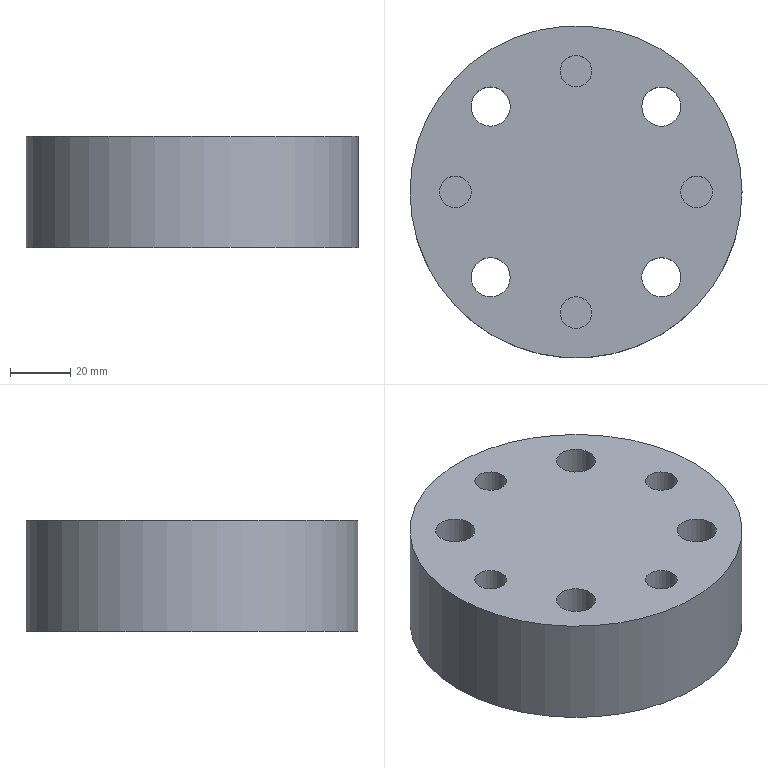Part | NX | 1 solid | 15 faces | box 110 x 110 x 37 mm | volume 326783 mm3 | cylinder 9 | plane 6 | commonest cylinder face diameters 10.5 x4 13 x4 110 x1
STEP:
#1=CARTESIAN_POINT('',(-28.284,34.784,-37.));
#2=VERTEX_POINT('',#1);
#3=CARTESIAN_POINT('',(-28.284,28.284,-37.));
#4=DIRECTION('',(0.,0.,1.));
#5=DIRECTION('',(0.,1.,0.));
#6=AXIS2_PLACEMENT_3D('',#3,#4,#5);
#7=CIRCLE('',#6,6.5);
#8=EDGE_CURVE('',#2,#2,#7,.T.);
#9=ORIENTED_EDGE('',*,*,#8,.F.);
#10=EDGE_LOOP('',(#9));
#11=FACE_BOUND('',#10,.T.);
#12=CARTESIAN_POINT('',(-28.284,34.784,0.));
#13=VERTEX_POINT('',#12);
#14=CARTESIAN_POINT('',(-28.284,28.284,0.));
#15=DIRECTION('',(0.,0.,1.));
#16=DIRECTION('',(0.,1.,0.));
#17=AXIS2_PLACEMENT_3D('',#14,#15,#16);
#18=CIRCLE('',#17,6.5);
#19=EDGE_CURVE('',#13,#13,#18,.T.);
#20=ORIENTED_EDGE('',*,*,#19,.T.);
#21=EDGE_LOOP('',(#20));
#22=FACE_BOUND('',#21,.T.);
#23=CARTESIAN_POINT('',(-28.284,28.284,-37.));
#24=DIRECTION('',(0.,0.,1.));
#25=DIRECTION('',(1.,0.,0.));
#26=AXIS2_PLACEMENT_3D('',#23,#24,#25);
#27=CYLINDRICAL_SURFACE('',#26,6.5);
#28=ADVANCED_FACE('',(#11,#22),#27,.F.);
#29=CARTESIAN_POINT('',(28.284,-34.784,-37.));
#30=VERTEX_POINT('',#29);
#31=CARTESIAN_POINT('',(28.284,-28.284,-37.));
#32=DIRECTION('',(0.,0.,1.));
#33=DIRECTION('',(0.,-1.,0.));
#34=AXIS2_PLACEMENT_3D('',#31,#32,#33);
#35=CIRCLE('',#34,6.5);
#36=EDGE_CURVE('',#30,#30,#35,.T.);
#37=ORIENTED_EDGE('',*,*,#36,.F.);
#38=EDGE_LOOP('',(#37));
#39=FACE_BOUND('',#38,.T.);
#40=CARTESIAN_POINT('',(28.284,-34.784,0.));
#41=VERTEX_POINT('',#40);
#42=CARTESIAN_POINT('',(28.284,-28.284,0.));
#43=DIRECTION('',(0.,0.,1.));
#44=DIRECTION('',(0.,-1.,0.));
#45=AXIS2_PLACEMENT_3D('',#42,#43,#44);
#46=CIRCLE('',#45,6.5);
#47=EDGE_CURVE('',#41,#41,#46,.T.);
#48=ORIENTED_EDGE('',*,*,#47,.T.);
#49=EDGE_LOOP('',(#48));
#50=FACE_BOUND('',#49,.T.);
#51=CARTESIAN_POINT('',(28.284,-28.284,-37.));
#52=DIRECTION('',(0.,0.,1.));
#53=DIRECTION('',(1.,0.,0.));
#54=AXIS2_PLACEMENT_3D('',#51,#52,#53);
#55=CYLINDRICAL_SURFACE('',#54,6.5);
#56=ADVANCED_FACE('',(#39,#50),#55,.F.);
#57=CARTESIAN_POINT('',(34.784,28.284,-37.));
#58=VERTEX_POINT('',#57);
#59=CARTESIAN_POINT('',(28.284,28.284,-37.));
#60=DIRECTION('',(0.,0.,1.));
#61=DIRECTION('',(1.,0.,0.));
#62=AXIS2_PLACEMENT_3D('',#59,#60,#61);
#63=CIRCLE('',#62,6.5);
#64=EDGE_CURVE('',#58,#58,#63,.T.);
#65=ORIENTED_EDGE('',*,*,#64,.F.);
#66=EDGE_LOOP('',(#65));
#67=FACE_BOUND('',#66,.T.);
#68=CARTESIAN_POINT('',(34.784,28.284,0.));
#69=VERTEX_POINT('',#68);
#70=CARTESIAN_POINT('',(28.284,28.284,0.));
#71=DIRECTION('',(0.,0.,1.));
#72=DIRECTION('',(1.,0.,0.));
#73=AXIS2_PLACEMENT_3D('',#70,#71,#72);
#74=CIRCLE('',#73,6.5);
#75=EDGE_CURVE('',#69,#69,#74,.T.);
#76=ORIENTED_EDGE('',*,*,#75,.T.);
#77=EDGE_LOOP('',(#76));
#78=FACE_BOUND('',#77,.T.);
#79=CARTESIAN_POINT('',(28.284,28.284,-37.));
#80=DIRECTION('',(0.,0.,1.));
#81=DIRECTION('',(1.,0.,0.));
#82=AXIS2_PLACEMENT_3D('',#79,#80,#81);
#83=CYLINDRICAL_SURFACE('',#82,6.5);
#84=ADVANCED_FACE('',(#67,#78),#83,.F.);
#85=CARTESIAN_POINT('',(55.,0.,-37.));
#86=VERTEX_POINT('',#85);
#87=CARTESIAN_POINT('',(0.,0.,-37.));
#88=DIRECTION('',(0.,0.,1.));
#89=DIRECTION('',(1.,0.,0.));
#90=AXIS2_PLACEMENT_3D('',#87,#88,#89);
#91=CIRCLE('',#90,55.);
#92=EDGE_CURVE('',#86,#86,#91,.T.);
#93=ORIENTED_EDGE('',*,*,#92,.T.);
#94=EDGE_LOOP('',(#93));
#95=FACE_BOUND('',#94,.T.);
#96=CARTESIAN_POINT('',(55.,0.,0.));
#97=VERTEX_POINT('',#96);
#98=CARTESIAN_POINT('',(0.,0.,0.));
#99=DIRECTION('',(0.,0.,1.));
#100=DIRECTION('',(1.,0.,0.));
#101=AXIS2_PLACEMENT_3D('',#98,#99,#100);
#102=CIRCLE('',#101,55.);
#103=EDGE_CURVE('',#97,#97,#102,.T.);
#104=ORIENTED_EDGE('',*,*,#103,.F.);
#105=EDGE_LOOP('',(#104));
#106=FACE_BOUND('',#105,.T.);
#107=CARTESIAN_POINT('',(0.,0.,-37.));
#108=DIRECTION('',(0.,0.,1.));
#109=DIRECTION('',(1.,0.,0.));
#110=AXIS2_PLACEMENT_3D('',#107,#108,#109);
#111=CYLINDRICAL_SURFACE('',#110,55.);
#112=ADVANCED_FACE('',(#95,#106),#111,.T.);
#113=CARTESIAN_POINT('',(-34.784,-28.284,-37.));
#114=VERTEX_POINT('',#113);
#115=CARTESIAN_POINT('',(-28.284,-28.284,-37.));
#116=DIRECTION('',(0.,0.,1.));
#117=DIRECTION('',(-1.,0.,0.));
#118=AXIS2_PLACEMENT_3D('',#115,#116,#117);
#119=CIRCLE('',#118,6.5);
#120=EDGE_CURVE('',#114,#114,#119,.T.);
#121=ORIENTED_EDGE('',*,*,#120,.F.);
#122=EDGE_LOOP('',(#121));
#123=FACE_BOUND('',#122,.T.);
#124=CARTESIAN_POINT('',(-34.784,-28.284,0.));
#125=VERTEX_POINT('',#124);
#126=CARTESIAN_POINT('',(-28.284,-28.284,0.));
#127=DIRECTION('',(0.,0.,1.));
#128=DIRECTION('',(-1.,0.,0.));
#129=AXIS2_PLACEMENT_3D('',#126,#127,#128);
#130=CIRCLE('',#129,6.5);
#131=EDGE_CURVE('',#125,#125,#130,.T.);
#132=ORIENTED_EDGE('',*,*,#131,.T.);
#133=EDGE_LOOP('',(#132));
#134=FACE_BOUND('',#133,.T.);
#135=CARTESIAN_POINT('',(-28.284,-28.284,-37.));
#136=DIRECTION('',(0.,0.,1.));
#137=DIRECTION('',(1.,0.,0.));
#138=AXIS2_PLACEMENT_3D('',#135,#136,#137);
#139=CYLINDRICAL_SURFACE('',#138,6.5);
#140=ADVANCED_FACE('',(#123,#134),#139,.F.);
#141=ORIENTED_EDGE('',*,*,#92,.F.);
#142=EDGE_LOOP('',(#141));
#143=FACE_BOUND('',#142,.T.);
#144=ORIENTED_EDGE('',*,*,#64,.T.);
#145=EDGE_LOOP('',(#144));
#146=FACE_BOUND('',#145,.T.);
#147=ORIENTED_EDGE('',*,*,#36,.T.);
#148=EDGE_LOOP('',(#147));
#149=FACE_BOUND('',#148,.T.);
#150=ORIENTED_EDGE('',*,*,#8,.T.);
#151=EDGE_LOOP('',(#150));
#152=FACE_BOUND('',#151,.T.);
#153=ORIENTED_EDGE('',*,*,#120,.T.);
#154=EDGE_LOOP('',(#153));
#155=FACE_BOUND('',#154,.T.);
#156=CARTESIAN_POINT('',(14.142,14.142,-37.));
#157=DIRECTION('',(0.,0.,1.));
#158=DIRECTION('',(1.,0.,0.));
#159=AXIS2_PLACEMENT_3D('',#156,#157,#158);
#160=PLANE('',#159);
#161=ADVANCED_FACE('',(#143,#146,#149,#152,#155),#160,.F.);
#162=CARTESIAN_POINT('',(40.,-5.25,0.));
#163=VERTEX_POINT('',#162);
#164=CARTESIAN_POINT('',(40.,0.,0.));
#165=DIRECTION('',(0.,0.,1.));
#166=DIRECTION('',(0.,-1.,0.));
#167=AXIS2_PLACEMENT_3D('',#164,#165,#166);
#168=CIRCLE('',#167,5.25);
#169=EDGE_CURVE('',#163,#163,#168,.T.);
#170=ORIENTED_EDGE('',*,*,#169,.F.);
#171=EDGE_LOOP('',(#170));
#172=FACE_BOUND('',#171,.T.);
#173=CARTESIAN_POINT('',(5.25,40.,0.));
#174=VERTEX_POINT('',#173);
#175=CARTESIAN_POINT('',(0.,40.,0.));
#176=DIRECTION('',(0.,0.,1.));
#177=DIRECTION('',(1.,0.,0.));
#178=AXIS2_PLACEMENT_3D('',#175,#176,#177);
#179=CIRCLE('',#178,5.25);
#180=EDGE_CURVE('',#174,#174,#179,.T.);
#181=ORIENTED_EDGE('',*,*,#180,.F.);
#182=EDGE_LOOP('',(#181));
#183=FACE_BOUND('',#182,.T.);
#184=CARTESIAN_POINT('',(-5.25,-40.,0.));
#185=VERTEX_POINT('',#184);
#186=CARTESIAN_POINT('',(0.,-40.,0.));
#187=DIRECTION('',(0.,0.,1.));
#188=DIRECTION('',(-1.,0.,0.));
#189=AXIS2_PLACEMENT_3D('',#186,#187,#188);
#190=CIRCLE('',#189,5.25);
#191=EDGE_CURVE('',#185,#185,#190,.T.);
#192=ORIENTED_EDGE('',*,*,#191,.F.);
#193=EDGE_LOOP('',(#192));
#194=FACE_BOUND('',#193,.T.);
#195=CARTESIAN_POINT('',(-40.,5.25,0.));
#196=VERTEX_POINT('',#195);
#197=CARTESIAN_POINT('',(-40.,0.,0.));
#198=DIRECTION('',(0.,0.,1.));
#199=DIRECTION('',(0.,1.,0.));
#200=AXIS2_PLACEMENT_3D('',#197,#198,#199);
#201=CIRCLE('',#200,5.25);
#202=EDGE_CURVE('',#196,#196,#201,.T.);
#203=ORIENTED_EDGE('',*,*,#202,.F.);
#204=EDGE_LOOP('',(#203));
#205=FACE_BOUND('',#204,.T.);
#206=ORIENTED_EDGE('',*,*,#103,.T.);
#207=EDGE_LOOP('',(#206));
#208=FACE_BOUND('',#207,.T.);
#209=ORIENTED_EDGE('',*,*,#75,.F.);
#210=EDGE_LOOP('',(#209));
#211=FACE_BOUND('',#210,.T.);
#212=ORIENTED_EDGE('',*,*,#47,.F.);
#213=EDGE_LOOP('',(#212));
#214=FACE_BOUND('',#213,.T.);
#215=ORIENTED_EDGE('',*,*,#19,.F.);
#216=EDGE_LOOP('',(#215));
#217=FACE_BOUND('',#216,.T.);
#218=ORIENTED_EDGE('',*,*,#131,.F.);
#219=EDGE_LOOP('',(#218));
#220=FACE_BOUND('',#219,.T.);
#221=CARTESIAN_POINT('',(14.142,14.142,0.));
#222=DIRECTION('',(0.,0.,1.));
#223=DIRECTION('',(1.,0.,0.));
#224=AXIS2_PLACEMENT_3D('',#221,#222,#223);
#225=PLANE('',#224);
#226=ADVANCED_FACE('',(#172,#183,#194,#205,#208,#211,#214,#217,#220),#225,.T.);
#227=CARTESIAN_POINT('',(-40.,5.25,-15.));
#228=VERTEX_POINT('',#227);
#229=CARTESIAN_POINT('',(-40.,0.,-15.));
#230=DIRECTION('',(0.,0.,1.));
#231=DIRECTION('',(0.,1.,0.));
#232=AXIS2_PLACEMENT_3D('',#229,#230,#231);
#233=CIRCLE('',#232,5.25);
#234=EDGE_CURVE('',#228,#228,#233,.F.);
#235=ORIENTED_EDGE('',*,*,#234,.T.);
#236=EDGE_LOOP('',(#235));
#237=FACE_BOUND('',#236,.T.);
#238=ORIENTED_EDGE('',*,*,#202,.T.);
#239=EDGE_LOOP('',(#238));
#240=FACE_BOUND('',#239,.T.);
#241=CARTESIAN_POINT('',(-40.,0.,-15.));
#242=DIRECTION('',(0.,0.,1.));
#243=DIRECTION('',(1.,0.,0.));
#244=AXIS2_PLACEMENT_3D('',#241,#242,#243);
#245=CYLINDRICAL_SURFACE('',#244,5.25);
#246=ADVANCED_FACE('',(#237,#240),#245,.F.);
#247=ORIENTED_EDGE('',*,*,#234,.F.);
#248=EDGE_LOOP('',(#247));
#249=FACE_BOUND('',#248,.T.);
#250=CARTESIAN_POINT('',(-40.,0.,-15.));
#251=DIRECTION('',(0.,0.,1.));
#252=DIRECTION('',(1.,0.,0.));
#253=AXIS2_PLACEMENT_3D('',#250,#251,#252);
#254=PLANE('',#253);
#255=ADVANCED_FACE('',(#249),#254,.T.);
#256=CARTESIAN_POINT('',(-5.25,-40.,-15.));
#257=VERTEX_POINT('',#256);
#258=CARTESIAN_POINT('',(0.,-40.,-15.));
#259=DIRECTION('',(0.,0.,1.));
#260=DIRECTION('',(-1.,0.,0.));
#261=AXIS2_PLACEMENT_3D('',#258,#259,#260);
#262=CIRCLE('',#261,5.25);
#263=EDGE_CURVE('',#257,#257,#262,.F.);
#264=ORIENTED_EDGE('',*,*,#263,.T.);
#265=EDGE_LOOP('',(#264));
#266=FACE_BOUND('',#265,.T.);
#267=ORIENTED_EDGE('',*,*,#191,.T.);
#268=EDGE_LOOP('',(#267));
#269=FACE_BOUND('',#268,.T.);
#270=CARTESIAN_POINT('',(0.,-40.,-15.));
#271=DIRECTION('',(0.,0.,1.));
#272=DIRECTION('',(1.,0.,0.));
#273=AXIS2_PLACEMENT_3D('',#270,#271,#272);
#274=CYLINDRICAL_SURFACE('',#273,5.25);
#275=ADVANCED_FACE('',(#266,#269),#274,.F.);
#276=ORIENTED_EDGE('',*,*,#263,.F.);
#277=EDGE_LOOP('',(#276));
#278=FACE_BOUND('',#277,.T.);
#279=CARTESIAN_POINT('',(0.,-40.,-15.));
#280=DIRECTION('',(0.,0.,1.));
#281=DIRECTION('',(1.,0.,0.));
#282=AXIS2_PLACEMENT_3D('',#279,#280,#281);
#283=PLANE('',#282);
#284=ADVANCED_FACE('',(#278),#283,.T.);
#285=CARTESIAN_POINT('',(5.25,40.,-15.));
#286=VERTEX_POINT('',#285);
#287=CARTESIAN_POINT('',(0.,40.,-15.));
#288=DIRECTION('',(0.,0.,1.));
#289=DIRECTION('',(1.,0.,0.));
#290=AXIS2_PLACEMENT_3D('',#287,#288,#289);
#291=CIRCLE('',#290,5.25);
#292=EDGE_CURVE('',#286,#286,#291,.F.);
#293=ORIENTED_EDGE('',*,*,#292,.T.);
#294=EDGE_LOOP('',(#293));
#295=FACE_BOUND('',#294,.T.);
#296=ORIENTED_EDGE('',*,*,#180,.T.);
#297=EDGE_LOOP('',(#296));
#298=FACE_BOUND('',#297,.T.);
#299=CARTESIAN_POINT('',(0.,40.,-15.));
#300=DIRECTION('',(0.,0.,1.));
#301=DIRECTION('',(1.,0.,0.));
#302=AXIS2_PLACEMENT_3D('',#299,#300,#301);
#303=CYLINDRICAL_SURFACE('',#302,5.25);
#304=ADVANCED_FACE('',(#295,#298),#303,.F.);
#305=ORIENTED_EDGE('',*,*,#292,.F.);
#306=EDGE_LOOP('',(#305));
#307=FACE_BOUND('',#306,.T.);
#308=CARTESIAN_POINT('',(0.,40.,-15.));
#309=DIRECTION('',(0.,0.,1.));
#310=DIRECTION('',(1.,0.,0.));
#311=AXIS2_PLACEMENT_3D('',#308,#309,#310);
#312=PLANE('',#311);
#313=ADVANCED_FACE('',(#307),#312,.T.);
#314=CARTESIAN_POINT('',(40.,-5.25,-15.));
#315=VERTEX_POINT('',#314);
#316=CARTESIAN_POINT('',(40.,0.,-15.));
#317=DIRECTION('',(0.,0.,1.));
#318=DIRECTION('',(0.,-1.,0.));
#319=AXIS2_PLACEMENT_3D('',#316,#317,#318);
#320=CIRCLE('',#319,5.25);
#321=EDGE_CURVE('',#315,#315,#320,.F.);
#322=ORIENTED_EDGE('',*,*,#321,.T.);
#323=EDGE_LOOP('',(#322));
#324=FACE_BOUND('',#323,.T.);
#325=ORIENTED_EDGE('',*,*,#169,.T.);
#326=EDGE_LOOP('',(#325));
#327=FACE_BOUND('',#326,.T.);
#328=CARTESIAN_POINT('',(40.,0.,-15.));
#329=DIRECTION('',(0.,0.,1.));
#330=DIRECTION('',(1.,0.,0.));
#331=AXIS2_PLACEMENT_3D('',#328,#329,#330);
#332=CYLINDRICAL_SURFACE('',#331,5.25);
#333=ADVANCED_FACE('',(#324,#327),#332,.F.);
#334=ORIENTED_EDGE('',*,*,#321,.F.);
#335=EDGE_LOOP('',(#334));
#336=FACE_BOUND('',#335,.T.);
#337=CARTESIAN_POINT('',(40.,0.,-15.));
#338=DIRECTION('',(0.,0.,1.));
#339=DIRECTION('',(1.,0.,0.));
#340=AXIS2_PLACEMENT_3D('',#337,#338,#339);
#341=PLANE('',#340);
#342=ADVANCED_FACE('',(#336),#341,.T.);
#343=CLOSED_SHELL('',(#28,#56,#84,#112,#140,#161,#226,#246,#255,#275,#284,#304,#313,#333,#342));
#344=MANIFOLD_SOLID_BREP('',#343);
#345=(LENGTH_UNIT()NAMED_UNIT(*)SI_UNIT(.MILLI.,.METRE.));
#346=UNCERTAINTY_MEASURE_WITH_UNIT(LENGTH_MEASURE(0.00001),#345,'','');
#347=(NAMED_UNIT(*)PLANE_ANGLE_UNIT()SI_UNIT($,.RADIAN.));
#348=(NAMED_UNIT(*)SI_UNIT($,.STERADIAN.)SOLID_ANGLE_UNIT());
#349=(GEOMETRIC_REPRESENTATION_CONTEXT(3)GLOBAL_UNCERTAINTY_ASSIGNED_CONTEXT((#346))GLOBAL_UNIT_ASSIGNED_CONTEXT((#345,#347,#348))REPRESENTATION_CONTEXT('',''));
#350=ADVANCED_BREP_SHAPE_REPRESENTATION('',(#344),#349);